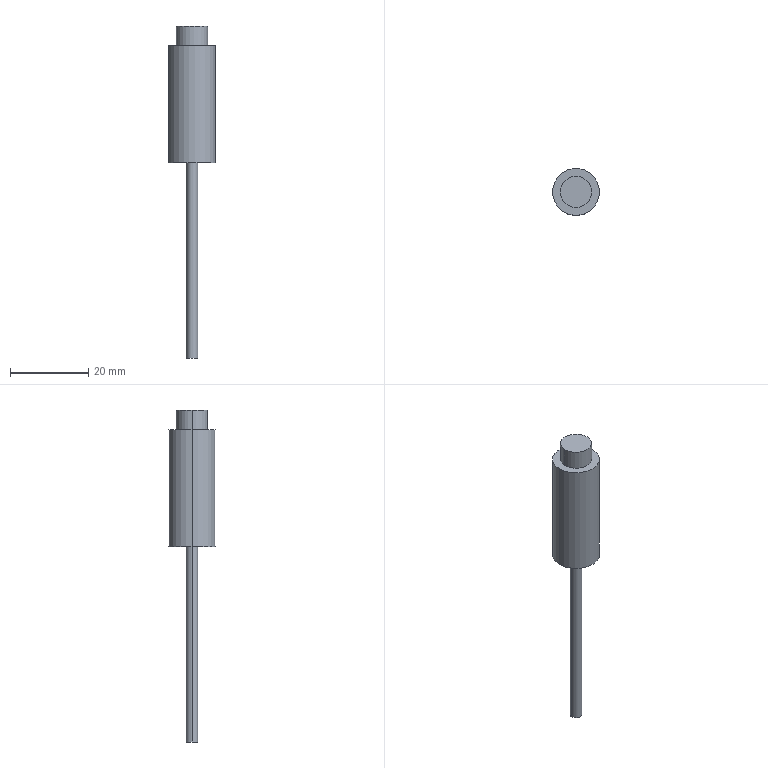Part | SolidWorks | features BaseBody 1 | 1 solid | 10 faces | box 12 x 12 x 85 mm | volume 3998 mm3 | cylinder 6 | plane 4 | commonest cylinder face diameters 3 x2 8 x2 12 x2
STEP:
#1=CARTESIAN_POINT('',(-6.,0.,30.));
#2=VERTEX_POINT('',#1);
#3=CARTESIAN_POINT('',(6.,0.,30.));
#4=VERTEX_POINT('',#3);
#5=CARTESIAN_POINT('',(0.,0.,30.));
#6=DIRECTION('',(0.,0.,-1.));
#7=DIRECTION('',(-1.,0.,0.));
#8=AXIS2_PLACEMENT_3D('',#5,#6,#7);
#9=CIRCLE('',#8,6.);
#10=EDGE_CURVE('',#2,#4,#9,.T.);
#11=ORIENTED_EDGE('',*,*,#10,.T.);
#12=CARTESIAN_POINT('',(6.,0.,0.));
#13=VERTEX_POINT('',#12);
#14=CARTESIAN_POINT('',(6.,0.,30.));
#15=DIRECTION('',(0.,0.,-1.));
#16=VECTOR('',#15,1000.);
#17=LINE('',#14,#16);
#18=EDGE_CURVE('',#4,#13,#17,.T.);
#19=ORIENTED_EDGE('',*,*,#18,.T.);
#20=CARTESIAN_POINT('',(-6.,0.,0.));
#21=VERTEX_POINT('',#20);
#22=CARTESIAN_POINT('',(0.,0.,0.));
#23=DIRECTION('',(0.,0.,1.));
#24=DIRECTION('',(-1.,0.,0.));
#25=AXIS2_PLACEMENT_3D('',#22,#23,#24);
#26=CIRCLE('',#25,6.);
#27=EDGE_CURVE('',#13,#21,#26,.T.);
#28=ORIENTED_EDGE('',*,*,#27,.T.);
#29=CARTESIAN_POINT('',(-6.,0.,30.));
#30=DIRECTION('',(0.,0.,-1.));
#31=VECTOR('',#30,1000.);
#32=LINE('',#29,#31);
#33=EDGE_CURVE('',#2,#21,#32,.T.);
#34=ORIENTED_EDGE('',*,*,#33,.F.);
#35=EDGE_LOOP('',(#11,#19,#28,#34));
#36=FACE_OUTER_BOUND('',#35,.T.);
#37=CARTESIAN_POINT('',(0.,0.,30.));
#38=DIRECTION('',(0.,0.,-1.));
#39=DIRECTION('',(-1.,0.,0.));
#40=AXIS2_PLACEMENT_3D('',#37,#38,#39);
#41=CYLINDRICAL_SURFACE('',#40,6.);
#42=ADVANCED_FACE('',(#36),#41,.T.);
#43=CARTESIAN_POINT('',(1.5,0.,-50.));
#44=VERTEX_POINT('',#43);
#45=CARTESIAN_POINT('',(-1.5,0.,-50.));
#46=VERTEX_POINT('',#45);
#47=CARTESIAN_POINT('',(0.,0.,-50.));
#48=DIRECTION('',(0.,0.,1.));
#49=DIRECTION('',(1.,0.,0.));
#50=AXIS2_PLACEMENT_3D('',#47,#48,#49);
#51=CIRCLE('',#50,1.5);
#52=EDGE_CURVE('',#44,#46,#51,.T.);
#53=ORIENTED_EDGE('',*,*,#52,.T.);
#54=CARTESIAN_POINT('',(-1.5,0.,0.));
#55=VERTEX_POINT('',#54);
#56=CARTESIAN_POINT('',(-1.5,0.,-50.));
#57=DIRECTION('',(0.,0.,1.));
#58=VECTOR('',#57,1000.);
#59=LINE('',#56,#58);
#60=EDGE_CURVE('',#46,#55,#59,.T.);
#61=ORIENTED_EDGE('',*,*,#60,.T.);
#62=CARTESIAN_POINT('',(1.5,0.,0.));
#63=VERTEX_POINT('',#62);
#64=CARTESIAN_POINT('',(0.,0.,0.));
#65=DIRECTION('',(0.,0.,-1.));
#66=DIRECTION('',(1.,0.,0.));
#67=AXIS2_PLACEMENT_3D('',#64,#65,#66);
#68=CIRCLE('',#67,1.5);
#69=EDGE_CURVE('',#55,#63,#68,.T.);
#70=ORIENTED_EDGE('',*,*,#69,.T.);
#71=CARTESIAN_POINT('',(1.5,0.,-50.));
#72=DIRECTION('',(0.,0.,1.));
#73=VECTOR('',#72,1000.);
#74=LINE('',#71,#73);
#75=EDGE_CURVE('',#44,#63,#74,.T.);
#76=ORIENTED_EDGE('',*,*,#75,.F.);
#77=EDGE_LOOP('',(#53,#61,#70,#76));
#78=FACE_OUTER_BOUND('',#77,.T.);
#79=CARTESIAN_POINT('',(0.,0.,-50.));
#80=DIRECTION('',(0.,0.,1.));
#81=DIRECTION('',(1.,0.,0.));
#82=AXIS2_PLACEMENT_3D('',#79,#80,#81);
#83=CYLINDRICAL_SURFACE('',#82,1.5);
#84=ADVANCED_FACE('',(#78),#83,.T.);
#85=CARTESIAN_POINT('',(-4.,0.,35.));
#86=VERTEX_POINT('',#85);
#87=CARTESIAN_POINT('',(4.,0.,35.));
#88=VERTEX_POINT('',#87);
#89=CARTESIAN_POINT('',(0.,0.,35.));
#90=DIRECTION('',(0.,0.,-1.));
#91=DIRECTION('',(-1.,0.,0.));
#92=AXIS2_PLACEMENT_3D('',#89,#90,#91);
#93=CIRCLE('',#92,4.);
#94=EDGE_CURVE('',#86,#88,#93,.T.);
#95=ORIENTED_EDGE('',*,*,#94,.T.);
#96=CARTESIAN_POINT('',(4.,0.,30.));
#97=VERTEX_POINT('',#96);
#98=CARTESIAN_POINT('',(4.,0.,35.));
#99=DIRECTION('',(0.,0.,-1.));
#100=VECTOR('',#99,1000.);
#101=LINE('',#98,#100);
#102=EDGE_CURVE('',#88,#97,#101,.T.);
#103=ORIENTED_EDGE('',*,*,#102,.T.);
#104=CARTESIAN_POINT('',(-4.,0.,30.));
#105=VERTEX_POINT('',#104);
#106=CARTESIAN_POINT('',(0.,0.,30.));
#107=DIRECTION('',(0.,0.,-1.));
#108=DIRECTION('',(-1.,0.,0.));
#109=AXIS2_PLACEMENT_3D('',#106,#107,#108);
#110=CIRCLE('',#109,4.);
#111=EDGE_CURVE('',#105,#97,#110,.T.);
#112=ORIENTED_EDGE('',*,*,#111,.F.);
#113=CARTESIAN_POINT('',(-4.,0.,35.));
#114=DIRECTION('',(0.,0.,-1.));
#115=VECTOR('',#114,1000.);
#116=LINE('',#113,#115);
#117=EDGE_CURVE('',#86,#105,#116,.T.);
#118=ORIENTED_EDGE('',*,*,#117,.F.);
#119=EDGE_LOOP('',(#95,#103,#112,#118));
#120=FACE_OUTER_BOUND('',#119,.T.);
#121=CARTESIAN_POINT('',(0.,0.,35.));
#122=DIRECTION('',(0.,0.,-1.));
#123=DIRECTION('',(-1.,0.,0.));
#124=AXIS2_PLACEMENT_3D('',#121,#122,#123);
#125=CYLINDRICAL_SURFACE('',#124,4.);
#126=ADVANCED_FACE('',(#120),#125,.T.);
#127=ORIENTED_EDGE('',*,*,#18,.F.);
#128=CARTESIAN_POINT('',(0.,0.,30.));
#129=DIRECTION('',(0.,0.,-1.));
#130=DIRECTION('',(-1.,0.,0.));
#131=AXIS2_PLACEMENT_3D('',#128,#129,#130);
#132=CIRCLE('',#131,6.);
#133=EDGE_CURVE('',#4,#2,#132,.T.);
#134=ORIENTED_EDGE('',*,*,#133,.T.);
#135=ORIENTED_EDGE('',*,*,#33,.T.);
#136=CARTESIAN_POINT('',(0.,0.,0.));
#137=DIRECTION('',(0.,0.,1.));
#138=DIRECTION('',(-1.,0.,0.));
#139=AXIS2_PLACEMENT_3D('',#136,#137,#138);
#140=CIRCLE('',#139,6.);
#141=EDGE_CURVE('',#21,#13,#140,.T.);
#142=ORIENTED_EDGE('',*,*,#141,.T.);
#143=EDGE_LOOP('',(#127,#134,#135,#142));
#144=FACE_OUTER_BOUND('',#143,.T.);
#145=CARTESIAN_POINT('',(0.,0.,30.));
#146=DIRECTION('',(0.,0.,-1.));
#147=DIRECTION('',(-1.,0.,0.));
#148=AXIS2_PLACEMENT_3D('',#145,#146,#147);
#149=CYLINDRICAL_SURFACE('',#148,6.);
#150=ADVANCED_FACE('',(#144),#149,.T.);
#151=ORIENTED_EDGE('',*,*,#141,.F.);
#152=ORIENTED_EDGE('',*,*,#27,.F.);
#153=EDGE_LOOP('',(#151,#152));
#154=FACE_OUTER_BOUND('',#153,.T.);
#155=CARTESIAN_POINT('',(0.,0.,0.));
#156=DIRECTION('',(0.,0.,-1.));
#157=DIRECTION('',(1.,0.,0.));
#158=AXIS2_PLACEMENT_3D('',#155,#156,#157);
#159=CIRCLE('',#158,1.5);
#160=EDGE_CURVE('',#63,#55,#159,.T.);
#161=ORIENTED_EDGE('',*,*,#160,.F.);
#162=ORIENTED_EDGE('',*,*,#69,.F.);
#163=EDGE_LOOP('',(#161,#162));
#164=FACE_BOUND('',#163,.T.);
#165=CARTESIAN_POINT('',(0.,0.,0.));
#166=DIRECTION('',(0.,0.,1.));
#167=DIRECTION('',(1.,0.,0.));
#168=AXIS2_PLACEMENT_3D('',#165,#166,#167);
#169=PLANE('',#168);
#170=ADVANCED_FACE('',(#154,#164),#169,.F.);
#171=ORIENTED_EDGE('',*,*,#10,.F.);
#172=ORIENTED_EDGE('',*,*,#133,.F.);
#173=EDGE_LOOP('',(#171,#172));
#174=FACE_OUTER_BOUND('',#173,.T.);
#175=ORIENTED_EDGE('',*,*,#111,.T.);
#176=CARTESIAN_POINT('',(0.,0.,30.));
#177=DIRECTION('',(0.,0.,-1.));
#178=DIRECTION('',(-1.,0.,0.));
#179=AXIS2_PLACEMENT_3D('',#176,#177,#178);
#180=CIRCLE('',#179,4.);
#181=EDGE_CURVE('',#97,#105,#180,.T.);
#182=ORIENTED_EDGE('',*,*,#181,.T.);
#183=EDGE_LOOP('',(#175,#182));
#184=FACE_BOUND('',#183,.T.);
#185=CARTESIAN_POINT('',(0.,0.,30.));
#186=DIRECTION('',(0.,0.,1.));
#187=DIRECTION('',(1.,0.,0.));
#188=AXIS2_PLACEMENT_3D('',#185,#186,#187);
#189=PLANE('',#188);
#190=ADVANCED_FACE('',(#174,#184),#189,.T.);
#191=ORIENTED_EDGE('',*,*,#60,.F.);
#192=CARTESIAN_POINT('',(0.,0.,-50.));
#193=DIRECTION('',(0.,0.,1.));
#194=DIRECTION('',(1.,0.,0.));
#195=AXIS2_PLACEMENT_3D('',#192,#193,#194);
#196=CIRCLE('',#195,1.5);
#197=EDGE_CURVE('',#46,#44,#196,.T.);
#198=ORIENTED_EDGE('',*,*,#197,.T.);
#199=ORIENTED_EDGE('',*,*,#75,.T.);
#200=ORIENTED_EDGE('',*,*,#160,.T.);
#201=EDGE_LOOP('',(#191,#198,#199,#200));
#202=FACE_OUTER_BOUND('',#201,.T.);
#203=CARTESIAN_POINT('',(0.,0.,-50.));
#204=DIRECTION('',(0.,0.,1.));
#205=DIRECTION('',(1.,0.,0.));
#206=AXIS2_PLACEMENT_3D('',#203,#204,#205);
#207=CYLINDRICAL_SURFACE('',#206,1.5);
#208=ADVANCED_FACE('',(#202),#207,.T.);
#209=ORIENTED_EDGE('',*,*,#102,.F.);
#210=CARTESIAN_POINT('',(0.,0.,35.));
#211=DIRECTION('',(0.,0.,-1.));
#212=DIRECTION('',(-1.,0.,0.));
#213=AXIS2_PLACEMENT_3D('',#210,#211,#212);
#214=CIRCLE('',#213,4.);
#215=EDGE_CURVE('',#88,#86,#214,.T.);
#216=ORIENTED_EDGE('',*,*,#215,.T.);
#217=ORIENTED_EDGE('',*,*,#117,.T.);
#218=ORIENTED_EDGE('',*,*,#181,.F.);
#219=EDGE_LOOP('',(#209,#216,#217,#218));
#220=FACE_OUTER_BOUND('',#219,.T.);
#221=CARTESIAN_POINT('',(0.,0.,35.));
#222=DIRECTION('',(0.,0.,-1.));
#223=DIRECTION('',(-1.,0.,0.));
#224=AXIS2_PLACEMENT_3D('',#221,#222,#223);
#225=CYLINDRICAL_SURFACE('',#224,4.);
#226=ADVANCED_FACE('',(#220),#225,.T.);
#227=ORIENTED_EDGE('',*,*,#52,.F.);
#228=ORIENTED_EDGE('',*,*,#197,.F.);
#229=EDGE_LOOP('',(#227,#228));
#230=FACE_OUTER_BOUND('',#229,.T.);
#231=CARTESIAN_POINT('',(0.,0.,-50.));
#232=DIRECTION('',(0.,0.,-1.));
#233=DIRECTION('',(-1.,0.,0.));
#234=AXIS2_PLACEMENT_3D('',#231,#232,#233);
#235=PLANE('',#234);
#236=ADVANCED_FACE('',(#230),#235,.T.);
#237=ORIENTED_EDGE('',*,*,#94,.F.);
#238=ORIENTED_EDGE('',*,*,#215,.F.);
#239=EDGE_LOOP('',(#237,#238));
#240=FACE_OUTER_BOUND('',#239,.T.);
#241=CARTESIAN_POINT('',(0.,0.,35.));
#242=DIRECTION('',(0.,0.,1.));
#243=DIRECTION('',(1.,0.,0.));
#244=AXIS2_PLACEMENT_3D('',#241,#242,#243);
#245=PLANE('',#244);
#246=ADVANCED_FACE('',(#240),#245,.T.);
#247=CLOSED_SHELL('',(#42,#84,#126,#150,#170,#190,#208,#226,#236,#246));
#248=MANIFOLD_SOLID_BREP('',#247);
#249=CARTESIAN_POINT('',(0.,0.,0.));
#250=DIRECTION('',(0.,0.,1.));
#251=DIRECTION('',(1.,0.,0.));
#252=AXIS2_PLACEMENT_3D('',#249,#250,#251);
#253=(LENGTH_UNIT()NAMED_UNIT(*)SI_UNIT(.MILLI.,.METRE.));
#254=UNCERTAINTY_MEASURE_WITH_UNIT(LENGTH_MEASURE(0.00001),#253,'','');
#255=(NAMED_UNIT(*)PLANE_ANGLE_UNIT()SI_UNIT($,.RADIAN.));
#256=(NAMED_UNIT(*)SI_UNIT($,.STERADIAN.)SOLID_ANGLE_UNIT());
#257=(GEOMETRIC_REPRESENTATION_CONTEXT(3)GLOBAL_UNCERTAINTY_ASSIGNED_CONTEXT((#254))GLOBAL_UNIT_ASSIGNED_CONTEXT((#253,#255,#256))REPRESENTATION_CONTEXT('',''));
#258=ADVANCED_BREP_SHAPE_REPRESENTATION('',(#248,#252),#257);